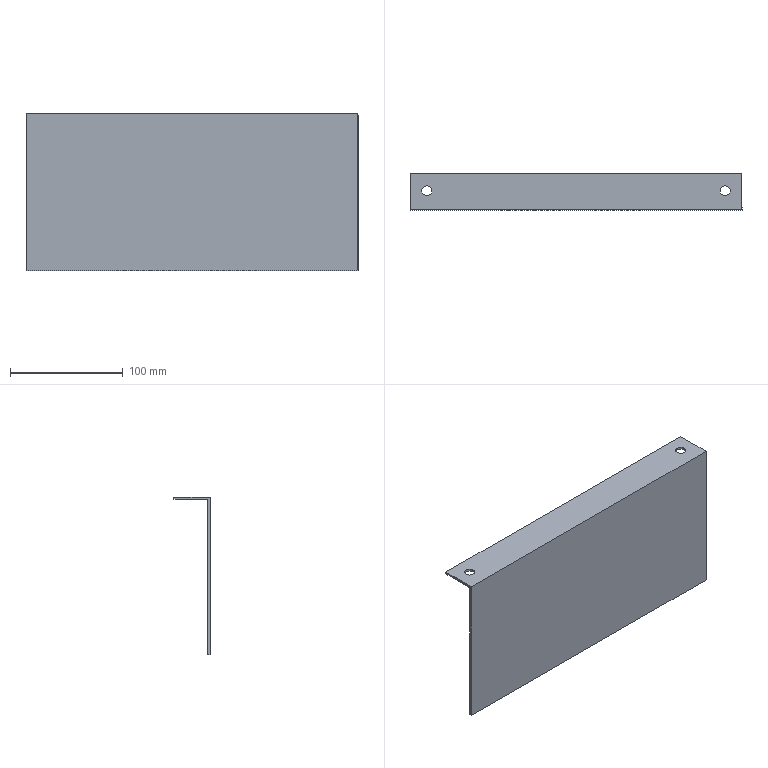Part | STEP file | lll_id2762_x_t | 1 solid | 10 faces | box 295 x 32 x 140 mm | volume 100046 mm3 | plane 8 | cylinder 2 | commonest cylinder face diameters 9 x2
STEP:
#1=CARTESIAN_POINT('',(554.935,441.,2.5));
#2=VERTEX_POINT('',#1);
#3=CARTESIAN_POINT('',(554.935,439.,2.5));
#4=VERTEX_POINT('',#3);
#5=CARTESIAN_POINT('',(554.935,441.,2.5));
#6=DIRECTION('',(0.,-1.,0.));
#7=VECTOR('',#6,1.);
#8=LINE('',#5,#7);
#9=EDGE_CURVE('',#2,#4,#8,.T.);
#10=ORIENTED_EDGE('',*,*,#9,.F.);
#11=CARTESIAN_POINT('',(849.935,441.,2.5));
#12=VERTEX_POINT('',#11);
#13=CARTESIAN_POINT('',(499.935,441.,2.5));
#14=DIRECTION('',(1.,0.,0.));
#15=VECTOR('',#14,1.);
#16=LINE('',#13,#15);
#17=EDGE_CURVE('',#2,#12,#16,.T.);
#18=ORIENTED_EDGE('',*,*,#17,.T.);
#19=CARTESIAN_POINT('',(849.935,439.,2.5));
#20=VERTEX_POINT('',#19);
#21=CARTESIAN_POINT('',(849.935,-45.,2.5));
#22=DIRECTION('',(0.,-1.,0.));
#23=VECTOR('',#22,1.);
#24=LINE('',#21,#23);
#25=EDGE_CURVE('',#12,#20,#24,.T.);
#26=ORIENTED_EDGE('',*,*,#25,.T.);
#27=CARTESIAN_POINT('',(499.935,439.,2.5));
#28=DIRECTION('',(1.,0.,0.));
#29=VECTOR('',#28,1.);
#30=LINE('',#27,#29);
#31=EDGE_CURVE('',#4,#20,#30,.T.);
#32=ORIENTED_EDGE('',*,*,#31,.F.);
#33=EDGE_LOOP('',(#10,#18,#26,#32));
#34=FACE_OUTER_BOUND('',#33,.T.);
#35=CARTESIAN_POINT('',(1692.435,-45.,2.5));
#36=DIRECTION('',(0.,0.,-1.));
#37=DIRECTION('',(-1.,0.,0.));
#38=AXIS2_PLACEMENT_3D('',#35,#36,#37);
#39=PLANE('',#38);
#40=ADVANCED_FACE('',(#34),#39,.T.);
#41=CARTESIAN_POINT('',(849.935,441.,140.5));
#42=VERTEX_POINT('',#41);
#43=CARTESIAN_POINT('',(554.935,441.,140.5));
#44=VERTEX_POINT('',#43);
#45=CARTESIAN_POINT('',(499.935,441.,140.5));
#46=DIRECTION('',(-1.,0.,0.));
#47=VECTOR('',#46,1.);
#48=LINE('',#45,#47);
#49=EDGE_CURVE('',#42,#44,#48,.T.);
#50=ORIENTED_EDGE('',*,*,#49,.F.);
#51=CARTESIAN_POINT('',(849.935,441.,-78.5));
#52=DIRECTION('',(0.,0.,1.));
#53=VECTOR('',#52,1.);
#54=LINE('',#51,#53);
#55=EDGE_CURVE('',#12,#42,#54,.T.);
#56=ORIENTED_EDGE('',*,*,#55,.F.);
#57=ORIENTED_EDGE('',*,*,#17,.F.);
#58=CARTESIAN_POINT('',(554.935,441.,142.5));
#59=DIRECTION('',(0.,0.,-1.));
#60=VECTOR('',#59,1.);
#61=LINE('',#58,#60);
#62=EDGE_CURVE('',#44,#2,#61,.T.);
#63=ORIENTED_EDGE('',*,*,#62,.F.);
#64=EDGE_LOOP('',(#50,#56,#57,#63));
#65=FACE_OUTER_BOUND('',#64,.T.);
#66=CARTESIAN_POINT('',(499.935,441.,-78.5));
#67=DIRECTION('',(0.,-1.,0.));
#68=DIRECTION('',(0.,0.,-1.));
#69=AXIS2_PLACEMENT_3D('',#66,#67,#68);
#70=PLANE('',#69);
#71=ADVANCED_FACE('',(#65),#70,.F.);
#72=CARTESIAN_POINT('',(554.935,439.,142.5));
#73=VERTEX_POINT('',#72);
#74=CARTESIAN_POINT('',(554.935,439.,-78.5));
#75=DIRECTION('',(0.,0.,-1.));
#76=VECTOR('',#75,1.);
#77=LINE('',#74,#76);
#78=EDGE_CURVE('',#73,#4,#77,.T.);
#79=ORIENTED_EDGE('',*,*,#78,.T.);
#80=ORIENTED_EDGE('',*,*,#31,.T.);
#81=CARTESIAN_POINT('',(849.935,439.,142.5));
#82=VERTEX_POINT('',#81);
#83=CARTESIAN_POINT('',(849.935,439.,-78.5));
#84=DIRECTION('',(0.,0.,1.));
#85=VECTOR('',#84,1.);
#86=LINE('',#83,#85);
#87=EDGE_CURVE('',#20,#82,#86,.T.);
#88=ORIENTED_EDGE('',*,*,#87,.T.);
#89=CARTESIAN_POINT('',(499.935,439.,142.5));
#90=DIRECTION('',(-1.,0.,0.));
#91=VECTOR('',#90,1.);
#92=LINE('',#89,#91);
#93=EDGE_CURVE('',#82,#73,#92,.T.);
#94=ORIENTED_EDGE('',*,*,#93,.T.);
#95=EDGE_LOOP('',(#79,#80,#88,#94));
#96=FACE_OUTER_BOUND('',#95,.T.);
#97=CARTESIAN_POINT('',(499.935,439.,-78.5));
#98=DIRECTION('',(0.,-1.,0.));
#99=DIRECTION('',(0.,0.,-1.));
#100=AXIS2_PLACEMENT_3D('',#97,#98,#99);
#101=PLANE('',#100);
#102=ADVANCED_FACE('',(#96),#101,.T.);
#103=ORIENTED_EDGE('',*,*,#9,.T.);
#104=ORIENTED_EDGE('',*,*,#78,.F.);
#105=CARTESIAN_POINT('',(554.935,471.,142.5));
#106=VERTEX_POINT('',#105);
#107=CARTESIAN_POINT('',(554.935,441.,142.5));
#108=DIRECTION('',(0.,-1.,0.));
#109=VECTOR('',#108,1.);
#110=LINE('',#107,#109);
#111=EDGE_CURVE('',#106,#73,#110,.T.);
#112=ORIENTED_EDGE('',*,*,#111,.F.);
#113=CARTESIAN_POINT('',(554.935,471.,140.5));
#114=VERTEX_POINT('',#113);
#115=CARTESIAN_POINT('',(554.935,471.,142.5));
#116=DIRECTION('',(0.,0.,-1.));
#117=VECTOR('',#116,1.);
#118=LINE('',#115,#117);
#119=EDGE_CURVE('',#106,#114,#118,.T.);
#120=ORIENTED_EDGE('',*,*,#119,.T.);
#121=CARTESIAN_POINT('',(554.935,441.,140.5));
#122=DIRECTION('',(0.,-1.,0.));
#123=VECTOR('',#122,1.);
#124=LINE('',#121,#123);
#125=EDGE_CURVE('',#114,#44,#124,.T.);
#126=ORIENTED_EDGE('',*,*,#125,.T.);
#127=ORIENTED_EDGE('',*,*,#62,.T.);
#128=EDGE_LOOP('',(#103,#104,#112,#120,#126,#127));
#129=FACE_OUTER_BOUND('',#128,.T.);
#130=CARTESIAN_POINT('',(554.935,441.,142.5));
#131=DIRECTION('',(-1.,0.,0.));
#132=DIRECTION('',(0.,0.,-1.));
#133=AXIS2_PLACEMENT_3D('',#130,#131,#132);
#134=PLANE('',#133);
#135=ADVANCED_FACE('',(#129),#134,.T.);
#136=ORIENTED_EDGE('',*,*,#119,.F.);
#137=CARTESIAN_POINT('',(849.935,471.,142.5));
#138=VERTEX_POINT('',#137);
#139=CARTESIAN_POINT('',(499.935,471.,142.5));
#140=DIRECTION('',(-1.,0.,0.));
#141=VECTOR('',#140,1.);
#142=LINE('',#139,#141);
#143=EDGE_CURVE('',#138,#106,#142,.T.);
#144=ORIENTED_EDGE('',*,*,#143,.F.);
#145=CARTESIAN_POINT('',(849.935,471.,140.5));
#146=VERTEX_POINT('',#145);
#147=CARTESIAN_POINT('',(849.935,471.,142.5));
#148=DIRECTION('',(0.,0.,-1.));
#149=VECTOR('',#148,1.);
#150=LINE('',#147,#149);
#151=EDGE_CURVE('',#138,#146,#150,.T.);
#152=ORIENTED_EDGE('',*,*,#151,.T.);
#153=CARTESIAN_POINT('',(499.935,471.,140.5));
#154=DIRECTION('',(-1.,0.,0.));
#155=VECTOR('',#154,1.);
#156=LINE('',#153,#155);
#157=EDGE_CURVE('',#146,#114,#156,.T.);
#158=ORIENTED_EDGE('',*,*,#157,.T.);
#159=EDGE_LOOP('',(#136,#144,#152,#158));
#160=FACE_OUTER_BOUND('',#159,.T.);
#161=CARTESIAN_POINT('',(499.935,471.,142.5));
#162=DIRECTION('',(0.,1.,0.));
#163=DIRECTION('',(1.,0.,0.));
#164=AXIS2_PLACEMENT_3D('',#161,#162,#163);
#165=PLANE('',#164);
#166=ADVANCED_FACE('',(#160),#165,.T.);
#167=CARTESIAN_POINT('',(849.935,441.,142.5));
#168=DIRECTION('',(0.,-1.,0.));
#169=VECTOR('',#168,1.);
#170=LINE('',#167,#169);
#171=EDGE_CURVE('',#138,#82,#170,.T.);
#172=ORIENTED_EDGE('',*,*,#171,.T.);
#173=ORIENTED_EDGE('',*,*,#87,.F.);
#174=ORIENTED_EDGE('',*,*,#25,.F.);
#175=ORIENTED_EDGE('',*,*,#55,.T.);
#176=CARTESIAN_POINT('',(849.935,441.,140.5));
#177=DIRECTION('',(0.,-1.,0.));
#178=VECTOR('',#177,1.);
#179=LINE('',#176,#178);
#180=EDGE_CURVE('',#146,#42,#179,.T.);
#181=ORIENTED_EDGE('',*,*,#180,.F.);
#182=ORIENTED_EDGE('',*,*,#151,.F.);
#183=EDGE_LOOP('',(#172,#173,#174,#175,#181,#182));
#184=FACE_OUTER_BOUND('',#183,.T.);
#185=CARTESIAN_POINT('',(849.935,441.,-78.5));
#186=DIRECTION('',(-1.,0.,0.));
#187=DIRECTION('',(0.,0.,-1.));
#188=AXIS2_PLACEMENT_3D('',#185,#186,#187);
#189=PLANE('',#188);
#190=ADVANCED_FACE('',(#184),#189,.F.);
#191=CARTESIAN_POINT('',(830.435,456.,142.5));
#192=VERTEX_POINT('',#191);
#193=CARTESIAN_POINT('',(834.935,456.,142.5));
#194=DIRECTION('',(0.,0.,1.));
#195=DIRECTION('',(-1.,0.,0.));
#196=AXIS2_PLACEMENT_3D('',#193,#194,#195);
#197=CIRCLE('',#196,4.5);
#198=EDGE_CURVE('',#192,#192,#197,.T.);
#199=ORIENTED_EDGE('',*,*,#198,.T.);
#200=EDGE_LOOP('',(#199));
#201=FACE_BOUND('',#200,.T.);
#202=CARTESIAN_POINT('',(839.435,456.,140.5));
#203=VERTEX_POINT('',#202);
#204=CARTESIAN_POINT('',(834.935,456.,140.5));
#205=DIRECTION('',(0.,0.,1.));
#206=DIRECTION('',(1.,0.,0.));
#207=AXIS2_PLACEMENT_3D('',#204,#205,#206);
#208=CIRCLE('',#207,4.5);
#209=EDGE_CURVE('',#203,#203,#208,.T.);
#210=ORIENTED_EDGE('',*,*,#209,.F.);
#211=EDGE_LOOP('',(#210));
#212=FACE_BOUND('',#211,.T.);
#213=CARTESIAN_POINT('',(834.935,456.,140.5));
#214=DIRECTION('',(0.,0.,1.));
#215=DIRECTION('',(1.,0.,0.));
#216=AXIS2_PLACEMENT_3D('',#213,#214,#215);
#217=CYLINDRICAL_SURFACE('',#216,4.5);
#218=ADVANCED_FACE('',(#201,#212),#217,.F.);
#219=CARTESIAN_POINT('',(565.435,456.,142.5));
#220=VERTEX_POINT('',#219);
#221=CARTESIAN_POINT('',(569.935,456.,142.5));
#222=DIRECTION('',(0.,0.,1.));
#223=DIRECTION('',(-1.,0.,0.));
#224=AXIS2_PLACEMENT_3D('',#221,#222,#223);
#225=CIRCLE('',#224,4.5);
#226=EDGE_CURVE('',#220,#220,#225,.T.);
#227=ORIENTED_EDGE('',*,*,#226,.T.);
#228=EDGE_LOOP('',(#227));
#229=FACE_BOUND('',#228,.T.);
#230=CARTESIAN_POINT('',(565.435,456.,140.5));
#231=VERTEX_POINT('',#230);
#232=CARTESIAN_POINT('',(569.935,456.,140.5));
#233=DIRECTION('',(0.,0.,1.));
#234=DIRECTION('',(-1.,0.,0.));
#235=AXIS2_PLACEMENT_3D('',#232,#233,#234);
#236=CIRCLE('',#235,4.5);
#237=EDGE_CURVE('',#231,#231,#236,.T.);
#238=ORIENTED_EDGE('',*,*,#237,.F.);
#239=EDGE_LOOP('',(#238));
#240=FACE_BOUND('',#239,.T.);
#241=CARTESIAN_POINT('',(569.935,456.,140.5));
#242=DIRECTION('',(0.,0.,1.));
#243=DIRECTION('',(-1.,0.,0.));
#244=AXIS2_PLACEMENT_3D('',#241,#242,#243);
#245=CYLINDRICAL_SURFACE('',#244,4.5);
#246=ADVANCED_FACE('',(#229,#240),#245,.F.);
#247=ORIENTED_EDGE('',*,*,#226,.F.);
#248=EDGE_LOOP('',(#247));
#249=FACE_BOUND('',#248,.T.);
#250=ORIENTED_EDGE('',*,*,#198,.F.);
#251=EDGE_LOOP('',(#250));
#252=FACE_BOUND('',#251,.T.);
#253=ORIENTED_EDGE('',*,*,#171,.F.);
#254=ORIENTED_EDGE('',*,*,#143,.T.);
#255=ORIENTED_EDGE('',*,*,#111,.T.);
#256=ORIENTED_EDGE('',*,*,#93,.F.);
#257=EDGE_LOOP('',(#253,#254,#255,#256));
#258=FACE_BOUND('',#257,.T.);
#259=CARTESIAN_POINT('',(499.935,441.,142.5));
#260=DIRECTION('',(0.,0.,-1.));
#261=DIRECTION('',(1.,0.,0.));
#262=AXIS2_PLACEMENT_3D('',#259,#260,#261);
#263=PLANE('',#262);
#264=ADVANCED_FACE('',(#249,#252,#258),#263,.F.);
#265=ORIENTED_EDGE('',*,*,#237,.T.);
#266=EDGE_LOOP('',(#265));
#267=FACE_BOUND('',#266,.T.);
#268=ORIENTED_EDGE('',*,*,#209,.T.);
#269=EDGE_LOOP('',(#268));
#270=FACE_BOUND('',#269,.T.);
#271=ORIENTED_EDGE('',*,*,#180,.T.);
#272=ORIENTED_EDGE('',*,*,#49,.T.);
#273=ORIENTED_EDGE('',*,*,#125,.F.);
#274=ORIENTED_EDGE('',*,*,#157,.F.);
#275=EDGE_LOOP('',(#271,#272,#273,#274));
#276=FACE_BOUND('',#275,.T.);
#277=CARTESIAN_POINT('',(499.935,441.,140.5));
#278=DIRECTION('',(0.,0.,-1.));
#279=DIRECTION('',(1.,0.,0.));
#280=AXIS2_PLACEMENT_3D('',#277,#278,#279);
#281=PLANE('',#280);
#282=ADVANCED_FACE('',(#267,#270,#276),#281,.T.);
#283=CLOSED_SHELL('',(#40,#71,#102,#135,#166,#190,#218,#246,#264,#282));
#284=MANIFOLD_SOLID_BREP('',#283);
#285=(LENGTH_UNIT()NAMED_UNIT(*)SI_UNIT(.MILLI.,.METRE.));
#286=UNCERTAINTY_MEASURE_WITH_UNIT(LENGTH_MEASURE(0.00002),#285,'','');
#287=(NAMED_UNIT(*)PLANE_ANGLE_UNIT()SI_UNIT($,.RADIAN.));
#288=PLANE_ANGLE_MEASURE_WITH_UNIT(PLANE_ANGLE_MEASURE(0.01745),#287);
#289=DIMENSIONAL_EXPONENTS(0.,0.,0.,0.,0.,0.,0.);
#290=(CONVERSION_BASED_UNIT('DEGREE',#288)NAMED_UNIT(#289)PLANE_ANGLE_UNIT());
#291=(NAMED_UNIT(*)SI_UNIT($,.STERADIAN.)SOLID_ANGLE_UNIT());
#292=(GEOMETRIC_REPRESENTATION_CONTEXT(3)GLOBAL_UNCERTAINTY_ASSIGNED_CONTEXT((#286))GLOBAL_UNIT_ASSIGNED_CONTEXT((#285,#290,#291))REPRESENTATION_CONTEXT('',''));
#293=ADVANCED_BREP_SHAPE_REPRESENTATION('',(#284),#292);